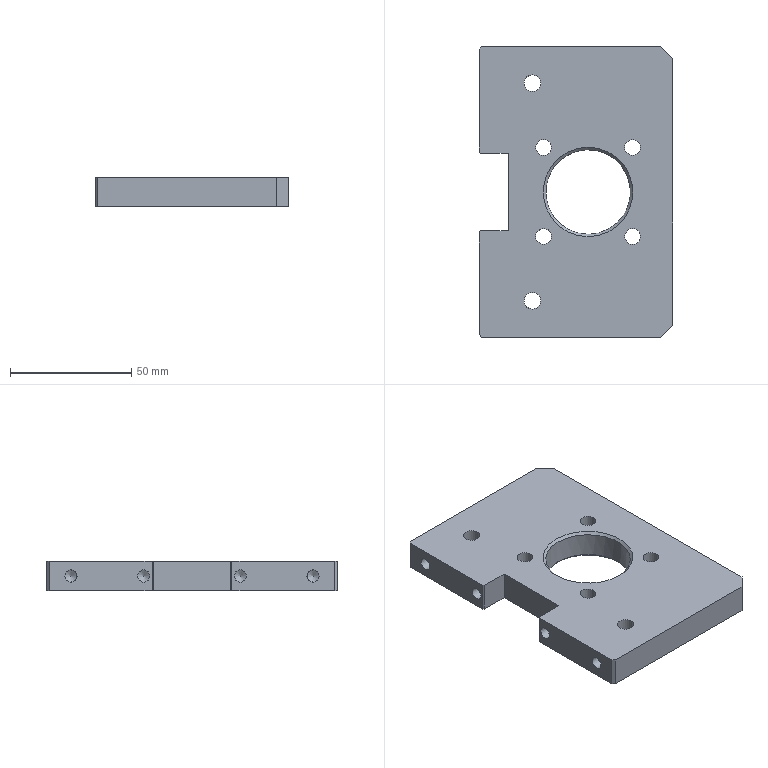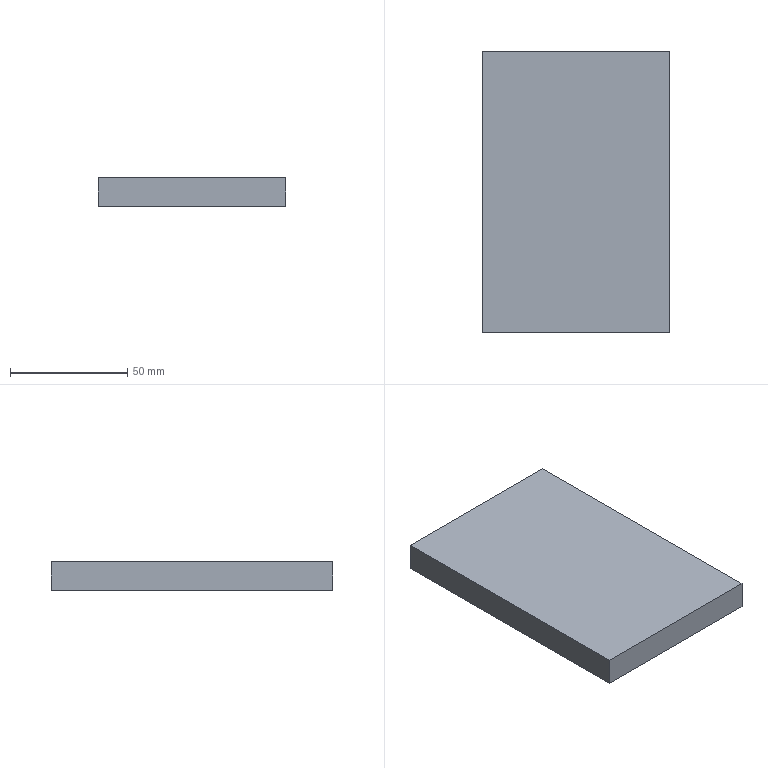CAM job | NX | 3+2 milling, drilling | part box 80 x 120 x 12 mm | stock box 80 x 120 x 12 mm
Tools:
number,name,description,diameter,corner_radius,flute_length,length,flutes
6,D8A45,Milling Tool-5 Parameters,8.0,0.0,50.0,75.0,2
14,5.0ZT,Drilling Tool,5.0,0.0,35.0,50.0,2
4,D10,Milling Tool-5 Parameters,10.0,0.0,50.0,75.0,2
15,6.8ZT,Drilling Tool,6.8,0.0,35.0,50.0,2
22,6.5ZT,Drilling Tool,6.5,0.0,35.0,50.0,2
Operations:
program,operation,operation_type,tool,method,geometry_group,spindle_rpm,surface_speed,feed_per_tooth,feed_cut,feed_plunge,cut_length_mm,path_length_mm,cut_time_min,machine_time_min
1,DRILLING,Operation,D8A45,METHOD,A,3500.0,65.0,0.0357,250.0,0.0,22.4,214.212,0.0896,0.1088
1,DRILLING_1,Operation,5.0ZT,METHOD,A,2000.0,26.0,0.05,200.0,0.0,97.773,364.959,0.4889,0.5156
1,FLOOR_WALL_1,VolumeBased25DMillingOperation,D10,METHOD,A,7000.0,219.0,0.2143,3000.0,1000.0,1384.099,1566.698,0.5299,0.5482
1,FLOOR_WALL_1_COPY,VolumeBased25DMillingOperation,D10,METHOD,A,7000.0,219.0,0.0857,1200.0,1000.0,220.422,331.922,0.1858,0.197
2,DRILLING_COPY,Operation,D8A45,METHOD,B,3500.0,65.0,0.0357,250.0,0.0,39.2,419.632,0.1568,0.1948
2,DRILLING_1_COPY,Operation,6.8ZT,METHOD,B,2000.0,26.0,0.05,200.0,0.0,37.086,227.222,0.1854,0.2044
2,DRILLING_1_COPY_COPY,Operation,6.5ZT,METHOD,B,2000.0,26.0,0.05,200.0,0.0,73.811,327.298,0.3691,0.3944
2,HOLE_MILLING,CylinderMilling,D10,METHOD,B,7000.0,0.0,0.0,2000.0,100.0,1636.382,1720.382,0.8182,0.8266
2,HOLE_MILLING_COPY,CylinderMilling,D10,METHOD,B,7000.0,0.0,0.0857,1200.0,100.0,388.176,459.676,0.3235,0.3306
2,PLANAR_MILL_COPY,PlanarMilling,D8A45,METHOD,B,7000.0,1495.0,0.0893,1250.0,100.0,643.805,1353.175,0.515,0.586